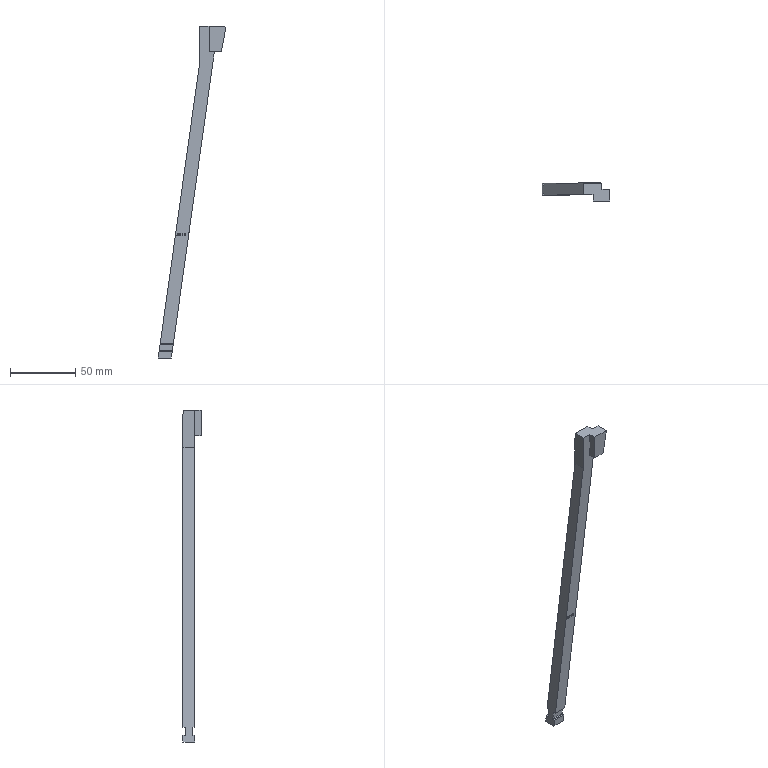Part | Creo | 1 solid | 101 faces | box 51.896 x 13.946 x 254.477 mm | volume 24800 mm3 | other 53 | plane 42 | cylinder 6 | commonest cylinder face diameters 1 x4 1.433 x1 22.6 x1